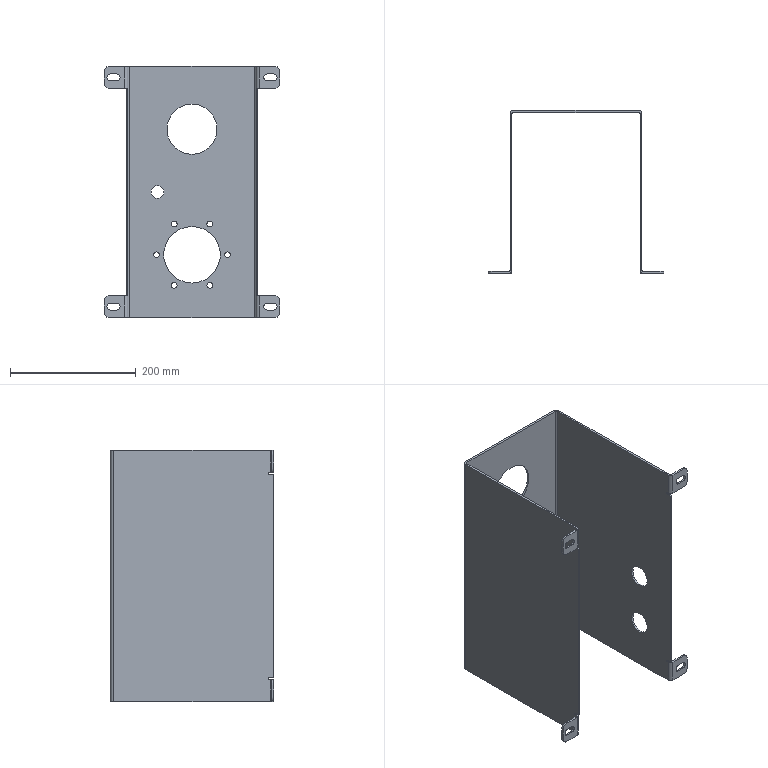Part | SolidWorks | features ICE 4, EdgeFlange 1, Fillet 1, FlatPattern 1, SMBaseFlange 1, SheetMetal 1, UnFold 1 | 1 solid | 124 faces | box 280 x 260 x 400 mm | volume 833549 mm3 | cylinder 62 | plane 62 | commonest cylinder face diameters 11 x18 9 x12 3 x8 16 x8 5 x6 35 x4